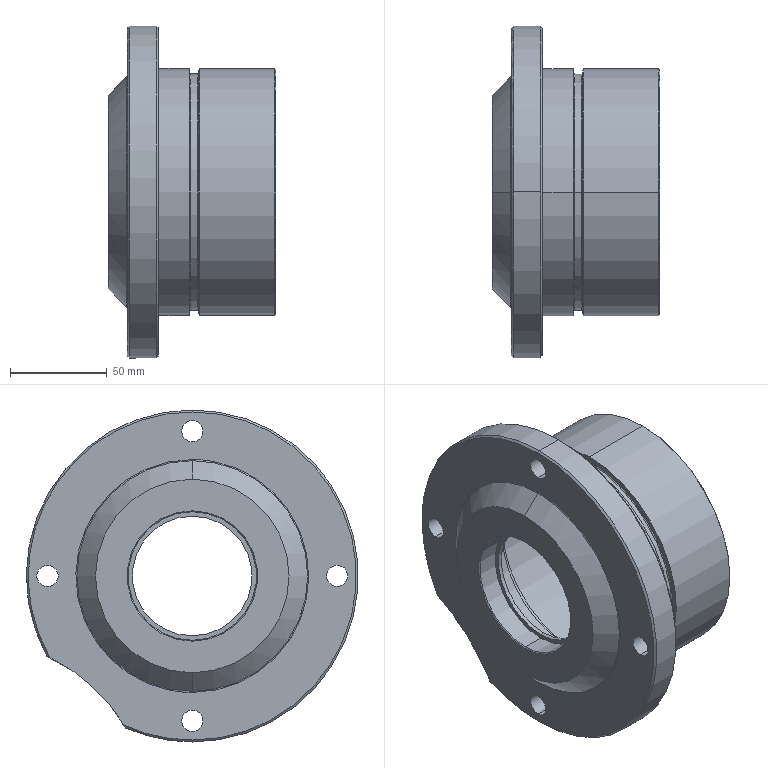Part | SolidWorks | features BaseBody 1 | 1 solid | 78 faces | box 86.84 x 172 x 172 mm | volume 547122 mm3 | cylinder 32 | spline 18 | cone 18 | plane 10 | commonest cylinder face diameters 11 x8 110 x4 128 x4 172 x3 62 x2 66.6 x2